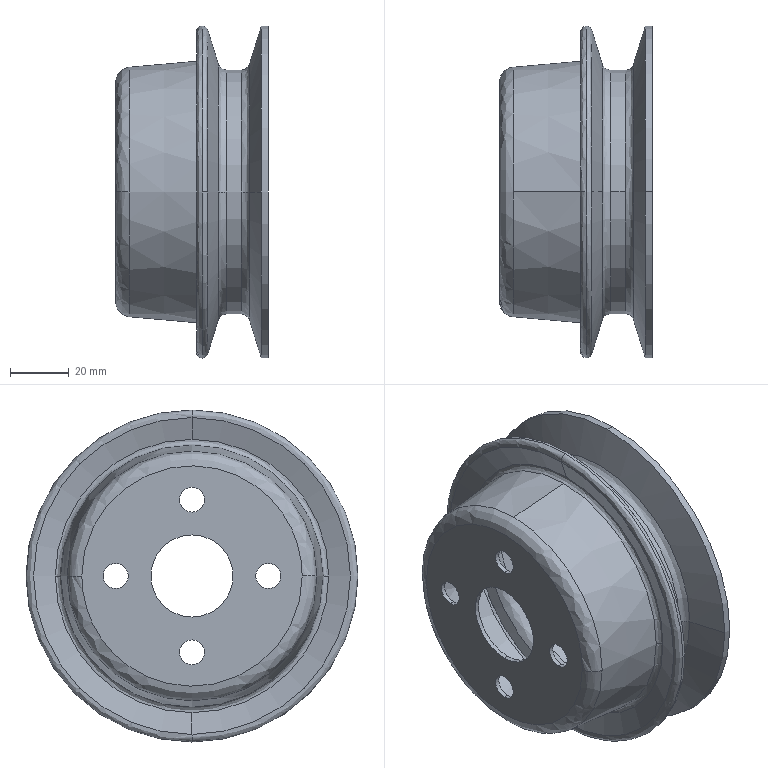Part | SolidWorks | features BaseBody 1 | 1 solid | 61 faces | box 51.997 x 113 x 113 mm | volume 43050 mm3 | spline 24 | cylinder 18 | cone 16 | plane 3 | commonest cylinder face diameters 8.5 x8 28 x2 80 x2 83 x2 110 x2 113 x2